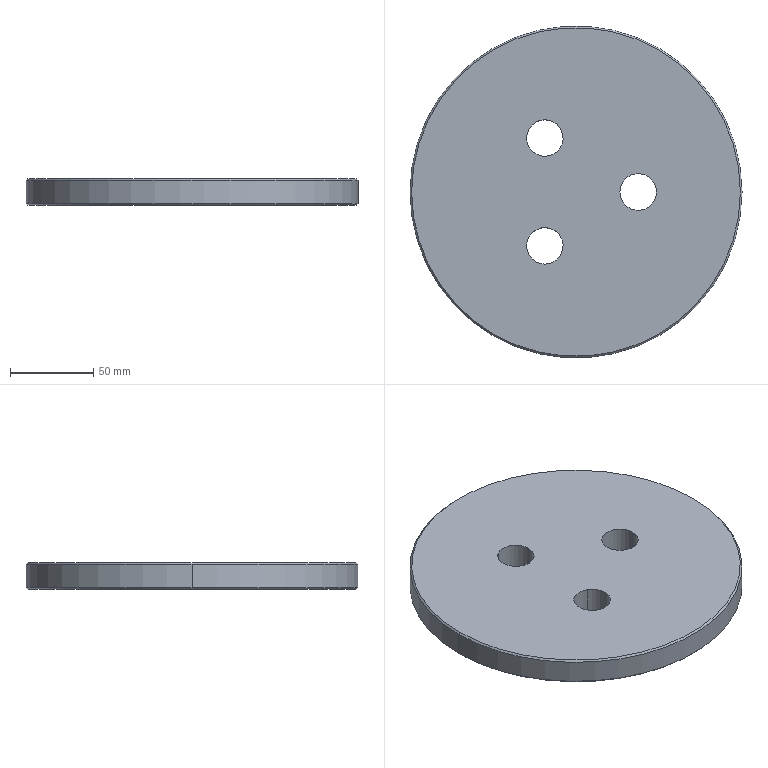Part | SolidWorks | features Chamfer 1, CirPattern 1, Extrusion 1, ICE 1 | 1 solid | 14 faces | box 200 x 200 x 16 mm | volume 483782 mm3 | cylinder 8 | cone 4 | plane 2 | commonest cylinder face diameters 22 x6 200 x2
STEP:
#1=CARTESIAN_POINT('',(99.,0.,16.));
#2=VERTEX_POINT('',#1);
#3=CARTESIAN_POINT('',(-99.,0.,16.));
#4=VERTEX_POINT('',#3);
#5=CARTESIAN_POINT('',(0.,0.,16.));
#6=DIRECTION('',(0.,0.,1.));
#7=DIRECTION('',(1.,0.,0.));
#8=AXIS2_PLACEMENT_3D('',#5,#6,#7);
#9=CIRCLE('',#8,99.);
#10=EDGE_CURVE('',#2,#4,#9,.T.);
#11=ORIENTED_EDGE('',*,*,#10,.F.);
#12=CARTESIAN_POINT('',(100.,0.,15.));
#13=VERTEX_POINT('',#12);
#14=CARTESIAN_POINT('',(99.,0.,16.));
#15=DIRECTION('',(0.7071,0.,-0.7071));
#16=VECTOR('',#15,1000.);
#17=LINE('',#14,#16);
#18=EDGE_CURVE('',#2,#13,#17,.T.);
#19=ORIENTED_EDGE('',*,*,#18,.T.);
#20=CARTESIAN_POINT('',(-100.,0.,15.));
#21=VERTEX_POINT('',#20);
#22=CARTESIAN_POINT('',(0.,0.,15.));
#23=DIRECTION('',(0.,0.,-1.));
#24=DIRECTION('',(1.,0.,0.));
#25=AXIS2_PLACEMENT_3D('',#22,#23,#24);
#26=CIRCLE('',#25,100.);
#27=EDGE_CURVE('',#21,#13,#26,.T.);
#28=ORIENTED_EDGE('',*,*,#27,.F.);
#29=CARTESIAN_POINT('',(-99.,0.,16.));
#30=DIRECTION('',(-0.7071,0.,-0.7071));
#31=VECTOR('',#30,1000.);
#32=LINE('',#29,#31);
#33=EDGE_CURVE('',#4,#21,#32,.T.);
#34=ORIENTED_EDGE('',*,*,#33,.F.);
#35=EDGE_LOOP('',(#11,#19,#28,#34));
#36=FACE_OUTER_BOUND('',#35,.T.);
#37=CARTESIAN_POINT('',(0.,0.,16.));
#38=DIRECTION('',(0.,0.,-1.));
#39=DIRECTION('',(-1.,0.,0.));
#40=AXIS2_PLACEMENT_3D('',#37,#38,#39);
#41=CONICAL_SURFACE('',#40,99.,0.7854);
#42=ADVANCED_FACE('',(#36),#41,.T.);
#43=CARTESIAN_POINT('',(-99.,0.,0.));
#44=VERTEX_POINT('',#43);
#45=CARTESIAN_POINT('',(99.,0.,0.));
#46=VERTEX_POINT('',#45);
#47=CARTESIAN_POINT('',(0.,0.,0.));
#48=DIRECTION('',(0.,0.,-1.));
#49=DIRECTION('',(1.,0.,0.));
#50=AXIS2_PLACEMENT_3D('',#47,#48,#49);
#51=CIRCLE('',#50,99.);
#52=EDGE_CURVE('',#44,#46,#51,.T.);
#53=ORIENTED_EDGE('',*,*,#52,.F.);
#54=CARTESIAN_POINT('',(-100.,0.,1.));
#55=VERTEX_POINT('',#54);
#56=CARTESIAN_POINT('',(-100.,0.,1.));
#57=DIRECTION('',(-0.7071,0.,0.7071));
#58=VECTOR('',#57,1000.);
#59=LINE('',#56,#58);
#60=EDGE_CURVE('',#44,#55,#59,.T.);
#61=ORIENTED_EDGE('',*,*,#60,.T.);
#62=CARTESIAN_POINT('',(100.,0.,1.));
#63=VERTEX_POINT('',#62);
#64=CARTESIAN_POINT('',(0.,0.,1.));
#65=DIRECTION('',(0.,0.,1.));
#66=DIRECTION('',(1.,0.,0.));
#67=AXIS2_PLACEMENT_3D('',#64,#65,#66);
#68=CIRCLE('',#67,100.);
#69=EDGE_CURVE('',#63,#55,#68,.T.);
#70=ORIENTED_EDGE('',*,*,#69,.F.);
#71=CARTESIAN_POINT('',(100.,0.,1.));
#72=DIRECTION('',(0.7071,0.,0.7071));
#73=VECTOR('',#72,1000.);
#74=LINE('',#71,#73);
#75=EDGE_CURVE('',#46,#63,#74,.T.);
#76=ORIENTED_EDGE('',*,*,#75,.F.);
#77=EDGE_LOOP('',(#53,#61,#70,#76));
#78=FACE_OUTER_BOUND('',#77,.T.);
#79=CARTESIAN_POINT('',(0.,0.,1.));
#80=DIRECTION('',(0.,0.,1.));
#81=DIRECTION('',(1.,0.,0.));
#82=AXIS2_PLACEMENT_3D('',#79,#80,#81);
#83=CONICAL_SURFACE('',#82,100.,0.7854);
#84=ADVANCED_FACE('',(#78),#83,.T.);
#85=CARTESIAN_POINT('',(-13.25,-22.95,0.));
#86=VERTEX_POINT('',#85);
#87=CARTESIAN_POINT('',(-24.25,-42.002,0.));
#88=VERTEX_POINT('',#87);
#89=CARTESIAN_POINT('',(-18.75,-32.476,0.));
#90=DIRECTION('',(0.,0.,1.));
#91=DIRECTION('',(-0.5,-0.866,0.));
#92=AXIS2_PLACEMENT_3D('',#89,#90,#91);
#93=CIRCLE('',#92,11.);
#94=EDGE_CURVE('',#86,#88,#93,.T.);
#95=ORIENTED_EDGE('',*,*,#94,.F.);
#96=CARTESIAN_POINT('',(-13.25,-22.95,16.));
#97=VERTEX_POINT('',#96);
#98=CARTESIAN_POINT('',(-13.25,-22.95,0.));
#99=DIRECTION('',(0.,0.,1.));
#100=VECTOR('',#99,1000.);
#101=LINE('',#98,#100);
#102=EDGE_CURVE('',#86,#97,#101,.T.);
#103=ORIENTED_EDGE('',*,*,#102,.T.);
#104=CARTESIAN_POINT('',(-24.25,-42.002,16.));
#105=VERTEX_POINT('',#104);
#106=CARTESIAN_POINT('',(-18.75,-32.476,16.));
#107=DIRECTION('',(0.,0.,1.));
#108=DIRECTION('',(-0.5,-0.866,0.));
#109=AXIS2_PLACEMENT_3D('',#106,#107,#108);
#110=CIRCLE('',#109,11.);
#111=EDGE_CURVE('',#97,#105,#110,.T.);
#112=ORIENTED_EDGE('',*,*,#111,.T.);
#113=CARTESIAN_POINT('',(-24.25,-42.002,0.));
#114=DIRECTION('',(0.,0.,1.));
#115=VECTOR('',#114,1000.);
#116=LINE('',#113,#115);
#117=EDGE_CURVE('',#88,#105,#116,.T.);
#118=ORIENTED_EDGE('',*,*,#117,.F.);
#119=EDGE_LOOP('',(#95,#103,#112,#118));
#120=FACE_OUTER_BOUND('',#119,.T.);
#121=CARTESIAN_POINT('',(-18.75,-32.476,0.));
#122=DIRECTION('',(0.,0.,1.));
#123=DIRECTION('',(-0.5,-0.866,0.));
#124=AXIS2_PLACEMENT_3D('',#121,#122,#123);
#125=CYLINDRICAL_SURFACE('',#124,11.);
#126=ADVANCED_FACE('',(#120),#125,.F.);
#127=CARTESIAN_POINT('',(-13.25,22.95,0.));
#128=VERTEX_POINT('',#127);
#129=CARTESIAN_POINT('',(-24.25,42.002,0.));
#130=VERTEX_POINT('',#129);
#131=CARTESIAN_POINT('',(-18.75,32.476,0.));
#132=DIRECTION('',(0.,0.,1.));
#133=DIRECTION('',(-0.5,0.866,0.));
#134=AXIS2_PLACEMENT_3D('',#131,#132,#133);
#135=CIRCLE('',#134,11.);
#136=EDGE_CURVE('',#128,#130,#135,.T.);
#137=ORIENTED_EDGE('',*,*,#136,.F.);
#138=CARTESIAN_POINT('',(-13.25,22.95,16.));
#139=VERTEX_POINT('',#138);
#140=CARTESIAN_POINT('',(-13.25,22.95,0.));
#141=DIRECTION('',(0.,0.,1.));
#142=VECTOR('',#141,1000.);
#143=LINE('',#140,#142);
#144=EDGE_CURVE('',#128,#139,#143,.T.);
#145=ORIENTED_EDGE('',*,*,#144,.T.);
#146=CARTESIAN_POINT('',(-24.25,42.002,16.));
#147=VERTEX_POINT('',#146);
#148=CARTESIAN_POINT('',(-18.75,32.476,16.));
#149=DIRECTION('',(0.,0.,1.));
#150=DIRECTION('',(-0.5,0.866,0.));
#151=AXIS2_PLACEMENT_3D('',#148,#149,#150);
#152=CIRCLE('',#151,11.);
#153=EDGE_CURVE('',#139,#147,#152,.T.);
#154=ORIENTED_EDGE('',*,*,#153,.T.);
#155=CARTESIAN_POINT('',(-24.25,42.002,0.));
#156=DIRECTION('',(0.,0.,1.));
#157=VECTOR('',#156,1000.);
#158=LINE('',#155,#157);
#159=EDGE_CURVE('',#130,#147,#158,.T.);
#160=ORIENTED_EDGE('',*,*,#159,.F.);
#161=EDGE_LOOP('',(#137,#145,#154,#160));
#162=FACE_OUTER_BOUND('',#161,.T.);
#163=CARTESIAN_POINT('',(-18.75,32.476,0.));
#164=DIRECTION('',(0.,0.,1.));
#165=DIRECTION('',(-0.5,0.866,0.));
#166=AXIS2_PLACEMENT_3D('',#163,#164,#165);
#167=CYLINDRICAL_SURFACE('',#166,11.);
#168=ADVANCED_FACE('',(#162),#167,.F.);
#169=CARTESIAN_POINT('',(26.5,0.,0.));
#170=VERTEX_POINT('',#169);
#171=CARTESIAN_POINT('',(48.5,0.,0.));
#172=VERTEX_POINT('',#171);
#173=CARTESIAN_POINT('',(37.5,0.,0.));
#174=DIRECTION('',(0.,0.,1.));
#175=DIRECTION('',(1.,0.,0.));
#176=AXIS2_PLACEMENT_3D('',#173,#174,#175);
#177=CIRCLE('',#176,11.);
#178=EDGE_CURVE('',#170,#172,#177,.T.);
#179=ORIENTED_EDGE('',*,*,#178,.F.);
#180=CARTESIAN_POINT('',(26.5,0.,16.));
#181=VERTEX_POINT('',#180);
#182=CARTESIAN_POINT('',(26.5,0.,0.));
#183=DIRECTION('',(0.,0.,1.));
#184=VECTOR('',#183,1000.);
#185=LINE('',#182,#184);
#186=EDGE_CURVE('',#170,#181,#185,.T.);
#187=ORIENTED_EDGE('',*,*,#186,.T.);
#188=CARTESIAN_POINT('',(48.5,0.,16.));
#189=VERTEX_POINT('',#188);
#190=CARTESIAN_POINT('',(37.5,0.,16.));
#191=DIRECTION('',(0.,0.,1.));
#192=DIRECTION('',(1.,0.,0.));
#193=AXIS2_PLACEMENT_3D('',#190,#191,#192);
#194=CIRCLE('',#193,11.);
#195=EDGE_CURVE('',#181,#189,#194,.T.);
#196=ORIENTED_EDGE('',*,*,#195,.T.);
#197=CARTESIAN_POINT('',(48.5,0.,0.));
#198=DIRECTION('',(0.,0.,1.));
#199=VECTOR('',#198,1000.);
#200=LINE('',#197,#199);
#201=EDGE_CURVE('',#172,#189,#200,.T.);
#202=ORIENTED_EDGE('',*,*,#201,.F.);
#203=EDGE_LOOP('',(#179,#187,#196,#202));
#204=FACE_OUTER_BOUND('',#203,.T.);
#205=CARTESIAN_POINT('',(37.5,0.,0.));
#206=DIRECTION('',(0.,0.,1.));
#207=DIRECTION('',(1.,0.,0.));
#208=AXIS2_PLACEMENT_3D('',#205,#206,#207);
#209=CYLINDRICAL_SURFACE('',#208,11.);
#210=ADVANCED_FACE('',(#204),#209,.F.);
#211=ORIENTED_EDGE('',*,*,#27,.T.);
#212=CARTESIAN_POINT('',(100.,0.,16.));
#213=DIRECTION('',(0.,0.,-1.));
#214=VECTOR('',#213,1000.);
#215=LINE('',#212,#214);
#216=EDGE_CURVE('',#13,#63,#215,.T.);
#217=ORIENTED_EDGE('',*,*,#216,.T.);
#218=ORIENTED_EDGE('',*,*,#69,.T.);
#219=CARTESIAN_POINT('',(-100.,0.,16.));
#220=DIRECTION('',(0.,0.,-1.));
#221=VECTOR('',#220,1000.);
#222=LINE('',#219,#221);
#223=EDGE_CURVE('',#21,#55,#222,.T.);
#224=ORIENTED_EDGE('',*,*,#223,.F.);
#225=EDGE_LOOP('',(#211,#217,#218,#224));
#226=FACE_OUTER_BOUND('',#225,.T.);
#227=CARTESIAN_POINT('',(0.,0.,16.));
#228=DIRECTION('',(0.,0.,-1.));
#229=DIRECTION('',(-1.,0.,0.));
#230=AXIS2_PLACEMENT_3D('',#227,#228,#229);
#231=CYLINDRICAL_SURFACE('',#230,100.);
#232=ADVANCED_FACE('',(#226),#231,.T.);
#233=ORIENTED_EDGE('',*,*,#216,.F.);
#234=CARTESIAN_POINT('',(0.,0.,15.));
#235=DIRECTION('',(0.,0.,-1.));
#236=DIRECTION('',(1.,0.,0.));
#237=AXIS2_PLACEMENT_3D('',#234,#235,#236);
#238=CIRCLE('',#237,100.);
#239=EDGE_CURVE('',#13,#21,#238,.T.);
#240=ORIENTED_EDGE('',*,*,#239,.T.);
#241=ORIENTED_EDGE('',*,*,#223,.T.);
#242=CARTESIAN_POINT('',(0.,0.,1.));
#243=DIRECTION('',(0.,0.,1.));
#244=DIRECTION('',(1.,0.,0.));
#245=AXIS2_PLACEMENT_3D('',#242,#243,#244);
#246=CIRCLE('',#245,100.);
#247=EDGE_CURVE('',#55,#63,#246,.T.);
#248=ORIENTED_EDGE('',*,*,#247,.T.);
#249=EDGE_LOOP('',(#233,#240,#241,#248));
#250=FACE_OUTER_BOUND('',#249,.T.);
#251=CARTESIAN_POINT('',(0.,0.,16.));
#252=DIRECTION('',(0.,0.,-1.));
#253=DIRECTION('',(-1.,0.,0.));
#254=AXIS2_PLACEMENT_3D('',#251,#252,#253);
#255=CYLINDRICAL_SURFACE('',#254,100.);
#256=ADVANCED_FACE('',(#250),#255,.T.);
#257=CARTESIAN_POINT('',(0.,0.,16.));
#258=DIRECTION('',(0.,0.,1.));
#259=DIRECTION('',(1.,0.,0.));
#260=AXIS2_PLACEMENT_3D('',#257,#258,#259);
#261=CIRCLE('',#260,99.);
#262=EDGE_CURVE('',#4,#2,#261,.T.);
#263=ORIENTED_EDGE('',*,*,#262,.T.);
#264=ORIENTED_EDGE('',*,*,#10,.T.);
#265=EDGE_LOOP('',(#263,#264));
#266=FACE_OUTER_BOUND('',#265,.T.);
#267=CARTESIAN_POINT('',(-18.75,-32.476,16.));
#268=DIRECTION('',(0.,0.,1.));
#269=DIRECTION('',(-0.5,-0.866,0.));
#270=AXIS2_PLACEMENT_3D('',#267,#268,#269);
#271=CIRCLE('',#270,11.);
#272=EDGE_CURVE('',#105,#97,#271,.T.);
#273=ORIENTED_EDGE('',*,*,#272,.F.);
#274=ORIENTED_EDGE('',*,*,#111,.F.);
#275=EDGE_LOOP('',(#273,#274));
#276=FACE_BOUND('',#275,.T.);
#277=CARTESIAN_POINT('',(-18.75,32.476,16.));
#278=DIRECTION('',(0.,0.,1.));
#279=DIRECTION('',(-0.5,0.866,0.));
#280=AXIS2_PLACEMENT_3D('',#277,#278,#279);
#281=CIRCLE('',#280,11.);
#282=EDGE_CURVE('',#147,#139,#281,.T.);
#283=ORIENTED_EDGE('',*,*,#282,.F.);
#284=ORIENTED_EDGE('',*,*,#153,.F.);
#285=EDGE_LOOP('',(#283,#284));
#286=FACE_BOUND('',#285,.T.);
#287=CARTESIAN_POINT('',(37.5,0.,16.));
#288=DIRECTION('',(0.,0.,1.));
#289=DIRECTION('',(1.,0.,0.));
#290=AXIS2_PLACEMENT_3D('',#287,#288,#289);
#291=CIRCLE('',#290,11.);
#292=EDGE_CURVE('',#189,#181,#291,.T.);
#293=ORIENTED_EDGE('',*,*,#292,.F.);
#294=ORIENTED_EDGE('',*,*,#195,.F.);
#295=EDGE_LOOP('',(#293,#294));
#296=FACE_BOUND('',#295,.T.);
#297=CARTESIAN_POINT('',(0.,0.,16.));
#298=DIRECTION('',(0.,0.,1.));
#299=DIRECTION('',(1.,0.,0.));
#300=AXIS2_PLACEMENT_3D('',#297,#298,#299);
#301=PLANE('',#300);
#302=ADVANCED_FACE('',(#266,#276,#286,#296),#301,.T.);
#303=CARTESIAN_POINT('',(0.,0.,0.));
#304=DIRECTION('',(0.,0.,-1.));
#305=DIRECTION('',(1.,0.,0.));
#306=AXIS2_PLACEMENT_3D('',#303,#304,#305);
#307=CIRCLE('',#306,99.);
#308=EDGE_CURVE('',#46,#44,#307,.T.);
#309=ORIENTED_EDGE('',*,*,#308,.T.);
#310=ORIENTED_EDGE('',*,*,#52,.T.);
#311=EDGE_LOOP('',(#309,#310));
#312=FACE_OUTER_BOUND('',#311,.T.);
#313=CARTESIAN_POINT('',(-18.75,-32.476,0.));
#314=DIRECTION('',(0.,0.,1.));
#315=DIRECTION('',(-0.5,-0.866,0.));
#316=AXIS2_PLACEMENT_3D('',#313,#314,#315);
#317=CIRCLE('',#316,11.);
#318=EDGE_CURVE('',#88,#86,#317,.T.);
#319=ORIENTED_EDGE('',*,*,#318,.T.);
#320=ORIENTED_EDGE('',*,*,#94,.T.);
#321=EDGE_LOOP('',(#319,#320));
#322=FACE_BOUND('',#321,.T.);
#323=CARTESIAN_POINT('',(-18.75,32.476,0.));
#324=DIRECTION('',(0.,0.,1.));
#325=DIRECTION('',(-0.5,0.866,0.));
#326=AXIS2_PLACEMENT_3D('',#323,#324,#325);
#327=CIRCLE('',#326,11.);
#328=EDGE_CURVE('',#130,#128,#327,.T.);
#329=ORIENTED_EDGE('',*,*,#328,.T.);
#330=ORIENTED_EDGE('',*,*,#136,.T.);
#331=EDGE_LOOP('',(#329,#330));
#332=FACE_BOUND('',#331,.T.);
#333=CARTESIAN_POINT('',(37.5,0.,0.));
#334=DIRECTION('',(0.,0.,1.));
#335=DIRECTION('',(1.,0.,0.));
#336=AXIS2_PLACEMENT_3D('',#333,#334,#335);
#337=CIRCLE('',#336,11.);
#338=EDGE_CURVE('',#172,#170,#337,.T.);
#339=ORIENTED_EDGE('',*,*,#338,.T.);
#340=ORIENTED_EDGE('',*,*,#178,.T.);
#341=EDGE_LOOP('',(#339,#340));
#342=FACE_BOUND('',#341,.T.);
#343=CARTESIAN_POINT('',(0.,0.,0.));
#344=DIRECTION('',(0.,0.,1.));
#345=DIRECTION('',(1.,0.,0.));
#346=AXIS2_PLACEMENT_3D('',#343,#344,#345);
#347=PLANE('',#346);
#348=ADVANCED_FACE('',(#312,#322,#332,#342),#347,.F.);
#349=ORIENTED_EDGE('',*,*,#186,.F.);
#350=ORIENTED_EDGE('',*,*,#338,.F.);
#351=ORIENTED_EDGE('',*,*,#201,.T.);
#352=ORIENTED_EDGE('',*,*,#292,.T.);
#353=EDGE_LOOP('',(#349,#350,#351,#352));
#354=FACE_OUTER_BOUND('',#353,.T.);
#355=CARTESIAN_POINT('',(37.5,0.,0.));
#356=DIRECTION('',(0.,0.,1.));
#357=DIRECTION('',(1.,0.,0.));
#358=AXIS2_PLACEMENT_3D('',#355,#356,#357);
#359=CYLINDRICAL_SURFACE('',#358,11.);
#360=ADVANCED_FACE('',(#354),#359,.F.);
#361=ORIENTED_EDGE('',*,*,#144,.F.);
#362=ORIENTED_EDGE('',*,*,#328,.F.);
#363=ORIENTED_EDGE('',*,*,#159,.T.);
#364=ORIENTED_EDGE('',*,*,#282,.T.);
#365=EDGE_LOOP('',(#361,#362,#363,#364));
#366=FACE_OUTER_BOUND('',#365,.T.);
#367=CARTESIAN_POINT('',(-18.75,32.476,0.));
#368=DIRECTION('',(0.,0.,1.));
#369=DIRECTION('',(-0.5,0.866,0.));
#370=AXIS2_PLACEMENT_3D('',#367,#368,#369);
#371=CYLINDRICAL_SURFACE('',#370,11.);
#372=ADVANCED_FACE('',(#366),#371,.F.);
#373=ORIENTED_EDGE('',*,*,#102,.F.);
#374=ORIENTED_EDGE('',*,*,#318,.F.);
#375=ORIENTED_EDGE('',*,*,#117,.T.);
#376=ORIENTED_EDGE('',*,*,#272,.T.);
#377=EDGE_LOOP('',(#373,#374,#375,#376));
#378=FACE_OUTER_BOUND('',#377,.T.);
#379=CARTESIAN_POINT('',(-18.75,-32.476,0.));
#380=DIRECTION('',(0.,0.,1.));
#381=DIRECTION('',(-0.5,-0.866,0.));
#382=AXIS2_PLACEMENT_3D('',#379,#380,#381);
#383=CYLINDRICAL_SURFACE('',#382,11.);
#384=ADVANCED_FACE('',(#378),#383,.F.);
#385=ORIENTED_EDGE('',*,*,#60,.F.);
#386=ORIENTED_EDGE('',*,*,#308,.F.);
#387=ORIENTED_EDGE('',*,*,#75,.T.);
#388=ORIENTED_EDGE('',*,*,#247,.F.);
#389=EDGE_LOOP('',(#385,#386,#387,#388));
#390=FACE_OUTER_BOUND('',#389,.T.);
#391=CARTESIAN_POINT('',(0.,0.,1.));
#392=DIRECTION('',(0.,0.,1.));
#393=DIRECTION('',(1.,0.,0.));
#394=AXIS2_PLACEMENT_3D('',#391,#392,#393);
#395=CONICAL_SURFACE('',#394,100.,0.7854);
#396=ADVANCED_FACE('',(#390),#395,.T.);
#397=ORIENTED_EDGE('',*,*,#18,.F.);
#398=ORIENTED_EDGE('',*,*,#262,.F.);
#399=ORIENTED_EDGE('',*,*,#33,.T.);
#400=ORIENTED_EDGE('',*,*,#239,.F.);
#401=EDGE_LOOP('',(#397,#398,#399,#400));
#402=FACE_OUTER_BOUND('',#401,.T.);
#403=CARTESIAN_POINT('',(0.,0.,16.));
#404=DIRECTION('',(0.,0.,-1.));
#405=DIRECTION('',(-1.,0.,0.));
#406=AXIS2_PLACEMENT_3D('',#403,#404,#405);
#407=CONICAL_SURFACE('',#406,99.,0.7854);
#408=ADVANCED_FACE('',(#402),#407,.T.);
#409=CLOSED_SHELL('',(#42,#84,#126,#168,#210,#232,#256,#302,#348,#360,#372,#384,#396,#408));
#410=MANIFOLD_SOLID_BREP('',#409);
#411=CARTESIAN_POINT('',(0.,0.,0.));
#412=DIRECTION('',(0.,0.,1.));
#413=DIRECTION('',(1.,0.,0.));
#414=AXIS2_PLACEMENT_3D('',#411,#412,#413);
#415=(LENGTH_UNIT()NAMED_UNIT(*)SI_UNIT(.MILLI.,.METRE.));
#416=UNCERTAINTY_MEASURE_WITH_UNIT(LENGTH_MEASURE(0.00001),#415,'','');
#417=(NAMED_UNIT(*)PLANE_ANGLE_UNIT()SI_UNIT($,.RADIAN.));
#418=(NAMED_UNIT(*)SI_UNIT($,.STERADIAN.)SOLID_ANGLE_UNIT());
#419=(GEOMETRIC_REPRESENTATION_CONTEXT(3)GLOBAL_UNCERTAINTY_ASSIGNED_CONTEXT((#416))GLOBAL_UNIT_ASSIGNED_CONTEXT((#415,#417,#418))REPRESENTATION_CONTEXT('',''));
#420=ADVANCED_BREP_SHAPE_REPRESENTATION('',(#410,#414),#419);